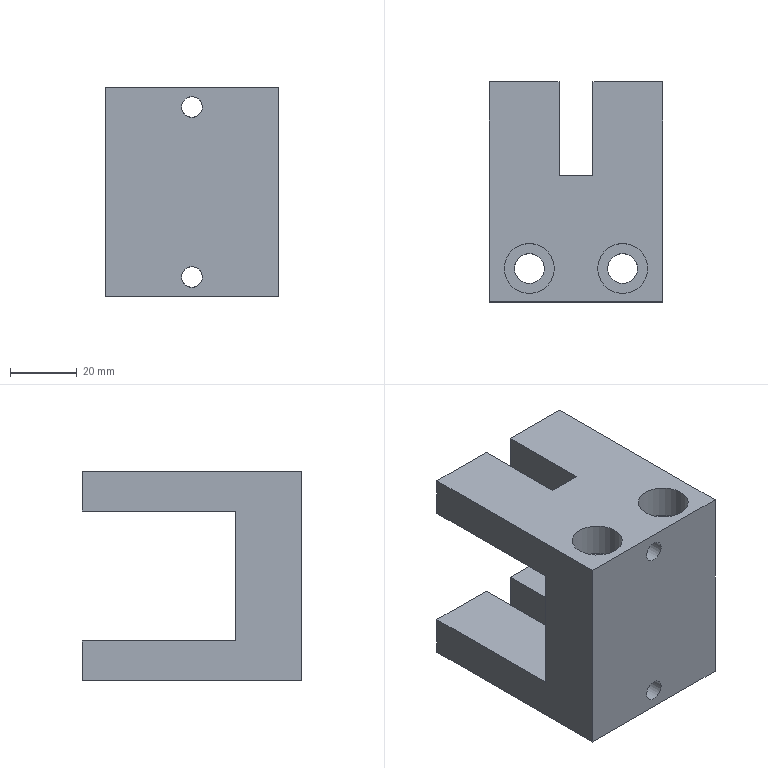Part | NX | 1 solid | 26 faces | box 52 x 66 x 63 mm | volume 103483 mm3 | plane 20 | cylinder 6 | commonest cylinder face diameters 6.2 x2 9 x2 15 x2
STEP:
#1=CARTESIAN_POINT('',(427.314,-68.057,-211.3));
#2=VERTEX_POINT('',#1);
#3=CARTESIAN_POINT('',(419.814,-68.057,-211.3));
#4=DIRECTION('',(0.,0.,1.));
#5=DIRECTION('',(1.,0.,0.));
#6=AXIS2_PLACEMENT_3D('',#3,#4,#5);
#7=CIRCLE('',#6,7.5);
#8=EDGE_CURVE('',#2,#2,#7,.T.);
#9=ORIENTED_EDGE('',*,*,#8,.T.);
#10=EDGE_LOOP('',(#9));
#11=FACE_BOUND('',#10,.T.);
#12=CARTESIAN_POINT('',(412.314,-68.057,-221.3));
#13=VERTEX_POINT('',#12);
#14=CARTESIAN_POINT('',(419.814,-68.057,-221.3));
#15=DIRECTION('',(0.,0.,1.));
#16=DIRECTION('',(-1.,0.,0.));
#17=AXIS2_PLACEMENT_3D('',#14,#15,#16);
#18=CIRCLE('',#17,7.5);
#19=EDGE_CURVE('',#13,#13,#18,.T.);
#20=ORIENTED_EDGE('',*,*,#19,.F.);
#21=EDGE_LOOP('',(#20));
#22=FACE_BOUND('',#21,.T.);
#23=CARTESIAN_POINT('',(419.814,-68.057,-211.3));
#24=DIRECTION('',(0.,0.,-1.));
#25=DIRECTION('',(1.,0.,0.));
#26=AXIS2_PLACEMENT_3D('',#23,#24,#25);
#27=CYLINDRICAL_SURFACE('',#26,7.5);
#28=ADVANCED_FACE('',(#11,#22),#27,.F.);
#29=ORIENTED_EDGE('',*,*,#19,.T.);
#30=EDGE_LOOP('',(#29));
#31=FACE_BOUND('',#30,.T.);
#32=CARTESIAN_POINT('',(415.314,-68.057,-221.3));
#33=VERTEX_POINT('',#32);
#34=CARTESIAN_POINT('',(419.814,-68.057,-221.3));
#35=DIRECTION('',(0.,0.,-1.));
#36=DIRECTION('',(-1.,0.,0.));
#37=AXIS2_PLACEMENT_3D('',#34,#35,#36);
#38=CIRCLE('',#37,4.5);
#39=EDGE_CURVE('',#33,#33,#38,.T.);
#40=ORIENTED_EDGE('',*,*,#39,.T.);
#41=EDGE_LOOP('',(#40));
#42=FACE_BOUND('',#41,.T.);
#43=CARTESIAN_POINT('',(391.814,-68.057,-221.3));
#44=DIRECTION('',(0.,0.,-1.));
#45=DIRECTION('',(1.,0.,0.));
#46=AXIS2_PLACEMENT_3D('',#43,#44,#45);
#47=PLANE('',#46);
#48=ADVANCED_FACE('',(#31,#42),#47,.F.);
#49=CARTESIAN_POINT('',(415.314,-68.057,-274.3));
#50=VERTEX_POINT('',#49);
#51=CARTESIAN_POINT('',(419.814,-68.057,-274.3));
#52=DIRECTION('',(0.,0.,1.));
#53=DIRECTION('',(-1.,0.,0.));
#54=AXIS2_PLACEMENT_3D('',#51,#52,#53);
#55=CIRCLE('',#54,4.5);
#56=EDGE_CURVE('',#50,#50,#55,.T.);
#57=ORIENTED_EDGE('',*,*,#56,.F.);
#58=EDGE_LOOP('',(#57));
#59=FACE_BOUND('',#58,.T.);
#60=ORIENTED_EDGE('',*,*,#39,.F.);
#61=EDGE_LOOP('',(#60));
#62=FACE_BOUND('',#61,.T.);
#63=CARTESIAN_POINT('',(419.814,-68.057,-211.3));
#64=DIRECTION('',(0.,0.,-1.));
#65=DIRECTION('',(1.,0.,0.));
#66=AXIS2_PLACEMENT_3D('',#63,#64,#65);
#67=CYLINDRICAL_SURFACE('',#66,4.5);
#68=ADVANCED_FACE('',(#59,#62),#67,.F.);
#69=CARTESIAN_POINT('',(384.314,-68.057,-211.3));
#70=VERTEX_POINT('',#69);
#71=CARTESIAN_POINT('',(391.814,-68.057,-211.3));
#72=DIRECTION('',(0.,0.,-1.));
#73=DIRECTION('',(-1.,0.,0.));
#74=AXIS2_PLACEMENT_3D('',#71,#72,#73);
#75=CIRCLE('',#74,7.5);
#76=EDGE_CURVE('',#70,#70,#75,.T.);
#77=ORIENTED_EDGE('',*,*,#76,.F.);
#78=EDGE_LOOP('',(#77));
#79=FACE_BOUND('',#78,.T.);
#80=CARTESIAN_POINT('',(384.314,-68.057,-221.3));
#81=VERTEX_POINT('',#80);
#82=CARTESIAN_POINT('',(391.814,-68.057,-221.3));
#83=DIRECTION('',(0.,0.,-1.));
#84=DIRECTION('',(-1.,0.,0.));
#85=AXIS2_PLACEMENT_3D('',#82,#83,#84);
#86=CIRCLE('',#85,7.5);
#87=EDGE_CURVE('',#81,#81,#86,.T.);
#88=ORIENTED_EDGE('',*,*,#87,.T.);
#89=EDGE_LOOP('',(#88));
#90=FACE_BOUND('',#89,.T.);
#91=CARTESIAN_POINT('',(391.814,-68.057,-211.3));
#92=DIRECTION('',(0.,0.,-1.));
#93=DIRECTION('',(-1.,0.,0.));
#94=AXIS2_PLACEMENT_3D('',#91,#92,#93);
#95=CYLINDRICAL_SURFACE('',#94,7.5);
#96=ADVANCED_FACE('',(#79,#90),#95,.F.);
#97=ORIENTED_EDGE('',*,*,#87,.F.);
#98=EDGE_LOOP('',(#97));
#99=FACE_BOUND('',#98,.T.);
#100=CARTESIAN_POINT('',(396.314,-68.057,-221.3));
#101=VERTEX_POINT('',#100);
#102=CARTESIAN_POINT('',(391.814,-68.057,-221.3));
#103=DIRECTION('',(0.,0.,1.));
#104=DIRECTION('',(1.,0.,0.));
#105=AXIS2_PLACEMENT_3D('',#102,#103,#104);
#106=CIRCLE('',#105,4.5);
#107=EDGE_CURVE('',#101,#101,#106,.T.);
#108=ORIENTED_EDGE('',*,*,#107,.F.);
#109=EDGE_LOOP('',(#108));
#110=FACE_BOUND('',#109,.T.);
#111=CARTESIAN_POINT('',(391.814,-68.057,-221.3));
#112=DIRECTION('',(0.,0.,-1.));
#113=DIRECTION('',(1.,0.,0.));
#114=AXIS2_PLACEMENT_3D('',#111,#112,#113);
#115=PLANE('',#114);
#116=ADVANCED_FACE('',(#99,#110),#115,.F.);
#117=CARTESIAN_POINT('',(387.314,-68.057,-274.3));
#118=VERTEX_POINT('',#117);
#119=CARTESIAN_POINT('',(391.814,-68.057,-274.3));
#120=DIRECTION('',(0.,0.,1.));
#121=DIRECTION('',(-1.,0.,0.));
#122=AXIS2_PLACEMENT_3D('',#119,#120,#121);
#123=CIRCLE('',#122,4.5);
#124=EDGE_CURVE('',#118,#118,#123,.T.);
#125=ORIENTED_EDGE('',*,*,#124,.F.);
#126=EDGE_LOOP('',(#125));
#127=FACE_BOUND('',#126,.T.);
#128=ORIENTED_EDGE('',*,*,#107,.T.);
#129=EDGE_LOOP('',(#128));
#130=FACE_BOUND('',#129,.T.);
#131=CARTESIAN_POINT('',(391.814,-68.057,-211.3));
#132=DIRECTION('',(0.,0.,-1.));
#133=DIRECTION('',(-1.,0.,0.));
#134=AXIS2_PLACEMENT_3D('',#131,#132,#133);
#135=CYLINDRICAL_SURFACE('',#134,4.5);
#136=ADVANCED_FACE('',(#127,#130),#135,.F.);
#137=CARTESIAN_POINT('',(431.814,-78.057,-274.3));
#138=VERTEX_POINT('',#137);
#139=CARTESIAN_POINT('',(431.814,-78.057,-211.3));
#140=VERTEX_POINT('',#139);
#141=CARTESIAN_POINT('',(431.814,-78.057,-217.3));
#142=DIRECTION('',(0.,0.,1.));
#143=VECTOR('',#142,1000.);
#144=LINE('',#141,#143);
#145=EDGE_CURVE('',#138,#140,#144,.T.);
#146=ORIENTED_EDGE('',*,*,#145,.F.);
#147=CARTESIAN_POINT('',(431.814,-12.057,-274.3));
#148=VERTEX_POINT('',#147);
#149=CARTESIAN_POINT('',(431.814,-34.899,-274.3));
#150=DIRECTION('',(0.,-1.,0.));
#151=VECTOR('',#150,1000.);
#152=LINE('',#149,#151);
#153=EDGE_CURVE('',#148,#138,#152,.T.);
#154=ORIENTED_EDGE('',*,*,#153,.F.);
#155=CARTESIAN_POINT('',(431.814,-12.057,-262.3));
#156=VERTEX_POINT('',#155);
#157=CARTESIAN_POINT('',(431.814,-12.057,-242.8));
#158=DIRECTION('',(0.,0.,1.));
#159=VECTOR('',#158,1000.);
#160=LINE('',#157,#159);
#161=EDGE_CURVE('',#148,#156,#160,.T.);
#162=ORIENTED_EDGE('',*,*,#161,.T.);
#163=CARTESIAN_POINT('',(431.814,-58.057,-262.3));
#164=VERTEX_POINT('',#163);
#165=CARTESIAN_POINT('',(431.814,-25.057,-262.3));
#166=DIRECTION('',(0.,1.,0.));
#167=VECTOR('',#166,1000.);
#168=LINE('',#165,#167);
#169=EDGE_CURVE('',#164,#156,#168,.T.);
#170=ORIENTED_EDGE('',*,*,#169,.F.);
#171=CARTESIAN_POINT('',(431.814,-58.057,-223.3));
#172=VERTEX_POINT('',#171);
#173=CARTESIAN_POINT('',(431.814,-58.057,-242.8));
#174=DIRECTION('',(0.,0.,-1.));
#175=VECTOR('',#174,1000.);
#176=LINE('',#173,#175);
#177=EDGE_CURVE('',#172,#164,#176,.T.);
#178=ORIENTED_EDGE('',*,*,#177,.F.);
#179=CARTESIAN_POINT('',(431.814,-12.057,-223.3));
#180=VERTEX_POINT('',#179);
#181=CARTESIAN_POINT('',(431.814,-26.107,-223.3));
#182=DIRECTION('',(0.,1.,0.));
#183=VECTOR('',#182,1000.);
#184=LINE('',#181,#183);
#185=EDGE_CURVE('',#172,#180,#184,.T.);
#186=ORIENTED_EDGE('',*,*,#185,.T.);
#187=CARTESIAN_POINT('',(431.814,-12.057,-211.3));
#188=VERTEX_POINT('',#187);
#189=CARTESIAN_POINT('',(431.814,-12.057,-242.8));
#190=DIRECTION('',(0.,0.,1.));
#191=VECTOR('',#190,1000.);
#192=LINE('',#189,#191);
#193=EDGE_CURVE('',#180,#188,#192,.T.);
#194=ORIENTED_EDGE('',*,*,#193,.T.);
#195=CARTESIAN_POINT('',(431.814,-34.899,-211.3));
#196=DIRECTION('',(0.,-1.,0.));
#197=VECTOR('',#196,1000.);
#198=LINE('',#195,#197);
#199=EDGE_CURVE('',#188,#140,#198,.T.);
#200=ORIENTED_EDGE('',*,*,#199,.T.);
#201=EDGE_LOOP('',(#146,#154,#162,#170,#178,#186,#194,#200));
#202=FACE_BOUND('',#201,.T.);
#203=CARTESIAN_POINT('',(431.814,-26.107,-217.3));
#204=DIRECTION('',(-1.,0.,0.));
#205=DIRECTION('',(0.,0.,-1.));
#206=AXIS2_PLACEMENT_3D('',#203,#204,#205);
#207=PLANE('',#206);
#208=ADVANCED_FACE('',(#202),#207,.F.);
#209=CARTESIAN_POINT('',(402.714,-40.157,-268.3));
#210=VERTEX_POINT('',#209);
#211=CARTESIAN_POINT('',(405.814,-40.157,-268.3));
#212=DIRECTION('',(0.,-1.,0.));
#213=DIRECTION('',(-1.,0.,0.));
#214=AXIS2_PLACEMENT_3D('',#211,#212,#213);
#215=CIRCLE('',#214,3.1);
#216=EDGE_CURVE('',#210,#210,#215,.T.);
#217=ORIENTED_EDGE('',*,*,#216,.F.);
#218=EDGE_LOOP('',(#217));
#219=FACE_BOUND('',#218,.T.);
#220=CARTESIAN_POINT('',(405.814,-78.057,-271.4));
#221=VERTEX_POINT('',#220);
#222=CARTESIAN_POINT('',(405.814,-78.057,-268.3));
#223=DIRECTION('',(0.,-1.,0.));
#224=DIRECTION('',(0.,0.,-1.));
#225=AXIS2_PLACEMENT_3D('',#222,#223,#224);
#226=CIRCLE('',#225,3.1);
#227=EDGE_CURVE('',#221,#221,#226,.T.);
#228=ORIENTED_EDGE('',*,*,#227,.T.);
#229=EDGE_LOOP('',(#228));
#230=FACE_BOUND('',#229,.T.);
#231=CARTESIAN_POINT('',(405.814,-30.057,-268.3));
#232=DIRECTION('',(0.,-1.,0.));
#233=DIRECTION('',(-1.,0.,0.));
#234=AXIS2_PLACEMENT_3D('',#231,#232,#233);
#235=CYLINDRICAL_SURFACE('',#234,3.1);
#236=ADVANCED_FACE('',(#219,#230),#235,.F.);
#237=CARTESIAN_POINT('',(402.714,-40.157,-217.3));
#238=VERTEX_POINT('',#237);
#239=CARTESIAN_POINT('',(405.814,-40.157,-217.3));
#240=DIRECTION('',(0.,-1.,0.));
#241=DIRECTION('',(-1.,0.,0.));
#242=AXIS2_PLACEMENT_3D('',#239,#240,#241);
#243=CIRCLE('',#242,3.1);
#244=EDGE_CURVE('',#238,#238,#243,.T.);
#245=ORIENTED_EDGE('',*,*,#244,.F.);
#246=EDGE_LOOP('',(#245));
#247=FACE_BOUND('',#246,.T.);
#248=CARTESIAN_POINT('',(405.814,-78.057,-220.4));
#249=VERTEX_POINT('',#248);
#250=CARTESIAN_POINT('',(405.814,-78.057,-217.3));
#251=DIRECTION('',(0.,-1.,0.));
#252=DIRECTION('',(0.,0.,-1.));
#253=AXIS2_PLACEMENT_3D('',#250,#251,#252);
#254=CIRCLE('',#253,3.1);
#255=EDGE_CURVE('',#249,#249,#254,.T.);
#256=ORIENTED_EDGE('',*,*,#255,.T.);
#257=EDGE_LOOP('',(#256));
#258=FACE_BOUND('',#257,.T.);
#259=CARTESIAN_POINT('',(405.814,-30.057,-217.3));
#260=DIRECTION('',(0.,-1.,0.));
#261=DIRECTION('',(-1.,0.,0.));
#262=AXIS2_PLACEMENT_3D('',#259,#260,#261);
#263=CYLINDRICAL_SURFACE('',#262,3.1);
#264=ADVANCED_FACE('',(#247,#258),#263,.F.);
#265=CARTESIAN_POINT('',(410.914,-40.157,-262.3));
#266=VERTEX_POINT('',#265);
#267=CARTESIAN_POINT('',(410.914,-40.157,-274.3));
#268=VERTEX_POINT('',#267);
#269=CARTESIAN_POINT('',(410.914,-40.157,-242.8));
#270=DIRECTION('',(0.,0.,-1.));
#271=VECTOR('',#270,1000.);
#272=LINE('',#269,#271);
#273=EDGE_CURVE('',#266,#268,#272,.T.);
#274=ORIENTED_EDGE('',*,*,#273,.T.);
#275=CARTESIAN_POINT('',(400.714,-40.157,-274.3));
#276=VERTEX_POINT('',#275);
#277=CARTESIAN_POINT('',(405.814,-40.157,-274.3));
#278=DIRECTION('',(1.,0.,0.));
#279=VECTOR('',#278,1000.);
#280=LINE('',#277,#279);
#281=EDGE_CURVE('',#276,#268,#280,.T.);
#282=ORIENTED_EDGE('',*,*,#281,.F.);
#283=CARTESIAN_POINT('',(400.714,-40.157,-262.3));
#284=VERTEX_POINT('',#283);
#285=CARTESIAN_POINT('',(400.714,-40.157,-242.8));
#286=DIRECTION('',(0.,0.,1.));
#287=VECTOR('',#286,1000.);
#288=LINE('',#285,#287);
#289=EDGE_CURVE('',#276,#284,#288,.T.);
#290=ORIENTED_EDGE('',*,*,#289,.T.);
#291=CARTESIAN_POINT('',(405.814,-40.157,-262.3));
#292=DIRECTION('',(-1.,0.,0.));
#293=VECTOR('',#292,1000.);
#294=LINE('',#291,#293);
#295=EDGE_CURVE('',#266,#284,#294,.T.);
#296=ORIENTED_EDGE('',*,*,#295,.F.);
#297=EDGE_LOOP('',(#274,#282,#290,#296));
#298=FACE_BOUND('',#297,.T.);
#299=ORIENTED_EDGE('',*,*,#216,.T.);
#300=EDGE_LOOP('',(#299));
#301=FACE_BOUND('',#300,.T.);
#302=CARTESIAN_POINT('',(400.714,-40.157,-242.8));
#303=DIRECTION('',(0.,-1.,0.));
#304=DIRECTION('',(-1.,0.,0.));
#305=AXIS2_PLACEMENT_3D('',#302,#303,#304);
#306=PLANE('',#305);
#307=ADVANCED_FACE('',(#298,#301),#306,.F.);
#308=ORIENTED_EDGE('',*,*,#289,.F.);
#309=CARTESIAN_POINT('',(400.714,-12.057,-274.3));
#310=VERTEX_POINT('',#309);
#311=CARTESIAN_POINT('',(400.714,-34.899,-274.3));
#312=DIRECTION('',(0.,-1.,0.));
#313=VECTOR('',#312,1000.);
#314=LINE('',#311,#313);
#315=EDGE_CURVE('',#310,#276,#314,.T.);
#316=ORIENTED_EDGE('',*,*,#315,.F.);
#317=CARTESIAN_POINT('',(400.714,-12.057,-262.3));
#318=VERTEX_POINT('',#317);
#319=CARTESIAN_POINT('',(400.714,-12.057,-242.8));
#320=DIRECTION('',(0.,0.,1.));
#321=VECTOR('',#320,1000.);
#322=LINE('',#319,#321);
#323=EDGE_CURVE('',#310,#318,#322,.T.);
#324=ORIENTED_EDGE('',*,*,#323,.T.);
#325=CARTESIAN_POINT('',(400.714,-25.057,-262.3));
#326=DIRECTION('',(0.,1.,0.));
#327=VECTOR('',#326,1000.);
#328=LINE('',#325,#327);
#329=EDGE_CURVE('',#284,#318,#328,.T.);
#330=ORIENTED_EDGE('',*,*,#329,.F.);
#331=EDGE_LOOP('',(#308,#316,#324,#330));
#332=FACE_BOUND('',#331,.T.);
#333=CARTESIAN_POINT('',(400.714,-25.057,-242.8));
#334=DIRECTION('',(-1.,0.,0.));
#335=DIRECTION('',(0.,1.,0.));
#336=AXIS2_PLACEMENT_3D('',#333,#334,#335);
#337=PLANE('',#336);
#338=ADVANCED_FACE('',(#332),#337,.F.);
#339=CARTESIAN_POINT('',(410.914,-12.057,-262.3));
#340=VERTEX_POINT('',#339);
#341=CARTESIAN_POINT('',(410.914,-12.057,-274.3));
#342=VERTEX_POINT('',#341);
#343=CARTESIAN_POINT('',(410.914,-12.057,-242.8));
#344=DIRECTION('',(0.,0.,-1.));
#345=VECTOR('',#344,1000.);
#346=LINE('',#343,#345);
#347=EDGE_CURVE('',#340,#342,#346,.T.);
#348=ORIENTED_EDGE('',*,*,#347,.T.);
#349=CARTESIAN_POINT('',(410.914,-34.899,-274.3));
#350=DIRECTION('',(0.,1.,0.));
#351=VECTOR('',#350,1000.);
#352=LINE('',#349,#351);
#353=EDGE_CURVE('',#268,#342,#352,.T.);
#354=ORIENTED_EDGE('',*,*,#353,.F.);
#355=ORIENTED_EDGE('',*,*,#273,.F.);
#356=CARTESIAN_POINT('',(410.914,-25.057,-262.3));
#357=DIRECTION('',(0.,-1.,0.));
#358=VECTOR('',#357,1000.);
#359=LINE('',#356,#358);
#360=EDGE_CURVE('',#340,#266,#359,.T.);
#361=ORIENTED_EDGE('',*,*,#360,.F.);
#362=EDGE_LOOP('',(#348,#354,#355,#361));
#363=FACE_BOUND('',#362,.T.);
#364=CARTESIAN_POINT('',(410.914,-25.057,-242.8));
#365=DIRECTION('',(1.,0.,0.));
#366=DIRECTION('',(0.,-1.,0.));
#367=AXIS2_PLACEMENT_3D('',#364,#365,#366);
#368=PLANE('',#367);
#369=ADVANCED_FACE('',(#363),#368,.F.);
#370=CARTESIAN_POINT('',(410.914,-40.157,-211.3));
#371=VERTEX_POINT('',#370);
#372=CARTESIAN_POINT('',(410.914,-12.057,-211.3));
#373=VERTEX_POINT('',#372);
#374=CARTESIAN_POINT('',(410.914,-34.899,-211.3));
#375=DIRECTION('',(0.,1.,0.));
#376=VECTOR('',#375,1000.);
#377=LINE('',#374,#376);
#378=EDGE_CURVE('',#371,#373,#377,.T.);
#379=ORIENTED_EDGE('',*,*,#378,.T.);
#380=CARTESIAN_POINT('',(410.914,-12.057,-223.3));
#381=VERTEX_POINT('',#380);
#382=CARTESIAN_POINT('',(410.914,-12.057,-242.8));
#383=DIRECTION('',(0.,0.,-1.));
#384=VECTOR('',#383,1000.);
#385=LINE('',#382,#384);
#386=EDGE_CURVE('',#373,#381,#385,.T.);
#387=ORIENTED_EDGE('',*,*,#386,.T.);
#388=CARTESIAN_POINT('',(410.914,-40.157,-223.3));
#389=VERTEX_POINT('',#388);
#390=CARTESIAN_POINT('',(410.914,-25.057,-223.3));
#391=DIRECTION('',(0.,1.,0.));
#392=VECTOR('',#391,1000.);
#393=LINE('',#390,#392);
#394=EDGE_CURVE('',#389,#381,#393,.T.);
#395=ORIENTED_EDGE('',*,*,#394,.F.);
#396=CARTESIAN_POINT('',(410.914,-40.157,-242.8));
#397=DIRECTION('',(0.,0.,-1.));
#398=VECTOR('',#397,1000.);
#399=LINE('',#396,#398);
#400=EDGE_CURVE('',#371,#389,#399,.T.);
#401=ORIENTED_EDGE('',*,*,#400,.F.);
#402=EDGE_LOOP('',(#379,#387,#395,#401));
#403=FACE_BOUND('',#402,.T.);
#404=CARTESIAN_POINT('',(410.914,-25.057,-242.8));
#405=DIRECTION('',(1.,0.,0.));
#406=DIRECTION('',(0.,-1.,0.));
#407=AXIS2_PLACEMENT_3D('',#404,#405,#406);
#408=PLANE('',#407);
#409=ADVANCED_FACE('',(#403),#408,.F.);
#410=CARTESIAN_POINT('',(400.714,-12.057,-211.3));
#411=VERTEX_POINT('',#410);
#412=CARTESIAN_POINT('',(400.714,-40.157,-211.3));
#413=VERTEX_POINT('',#412);
#414=CARTESIAN_POINT('',(400.714,-34.899,-211.3));
#415=DIRECTION('',(0.,-1.,0.));
#416=VECTOR('',#415,1000.);
#417=LINE('',#414,#416);
#418=EDGE_CURVE('',#411,#413,#417,.T.);
#419=ORIENTED_EDGE('',*,*,#418,.T.);
#420=CARTESIAN_POINT('',(400.714,-40.157,-223.3));
#421=VERTEX_POINT('',#420);
#422=CARTESIAN_POINT('',(400.714,-40.157,-242.8));
#423=DIRECTION('',(0.,0.,1.));
#424=VECTOR('',#423,1000.);
#425=LINE('',#422,#424);
#426=EDGE_CURVE('',#421,#413,#425,.T.);
#427=ORIENTED_EDGE('',*,*,#426,.F.);
#428=CARTESIAN_POINT('',(400.714,-12.057,-223.3));
#429=VERTEX_POINT('',#428);
#430=CARTESIAN_POINT('',(400.714,-25.057,-223.3));
#431=DIRECTION('',(0.,-1.,0.));
#432=VECTOR('',#431,1000.);
#433=LINE('',#430,#432);
#434=EDGE_CURVE('',#429,#421,#433,.T.);
#435=ORIENTED_EDGE('',*,*,#434,.F.);
#436=CARTESIAN_POINT('',(400.714,-12.057,-242.8));
#437=DIRECTION('',(0.,0.,1.));
#438=VECTOR('',#437,1000.);
#439=LINE('',#436,#438);
#440=EDGE_CURVE('',#429,#411,#439,.T.);
#441=ORIENTED_EDGE('',*,*,#440,.T.);
#442=EDGE_LOOP('',(#419,#427,#435,#441));
#443=FACE_BOUND('',#442,.T.);
#444=CARTESIAN_POINT('',(400.714,-25.057,-242.8));
#445=DIRECTION('',(-1.,0.,0.));
#446=DIRECTION('',(0.,1.,0.));
#447=AXIS2_PLACEMENT_3D('',#444,#445,#446);
#448=PLANE('',#447);
#449=ADVANCED_FACE('',(#443),#448,.F.);
#450=CARTESIAN_POINT('',(405.814,-40.157,-211.3));
#451=DIRECTION('',(1.,0.,0.));
#452=VECTOR('',#451,1000.);
#453=LINE('',#450,#452);
#454=EDGE_CURVE('',#413,#371,#453,.T.);
#455=ORIENTED_EDGE('',*,*,#454,.T.);
#456=ORIENTED_EDGE('',*,*,#400,.T.);
#457=CARTESIAN_POINT('',(405.814,-40.157,-223.3));
#458=DIRECTION('',(1.,0.,0.));
#459=VECTOR('',#458,1000.);
#460=LINE('',#457,#459);
#461=EDGE_CURVE('',#421,#389,#460,.T.);
#462=ORIENTED_EDGE('',*,*,#461,.F.);
#463=ORIENTED_EDGE('',*,*,#426,.T.);
#464=EDGE_LOOP('',(#455,#456,#462,#463));
#465=FACE_BOUND('',#464,.T.);
#466=ORIENTED_EDGE('',*,*,#244,.T.);
#467=EDGE_LOOP('',(#466));
#468=FACE_BOUND('',#467,.T.);
#469=CARTESIAN_POINT('',(400.714,-40.157,-242.8));
#470=DIRECTION('',(0.,-1.,0.));
#471=DIRECTION('',(-1.,0.,0.));
#472=AXIS2_PLACEMENT_3D('',#469,#470,#471);
#473=PLANE('',#472);
#474=ADVANCED_FACE('',(#465,#468),#473,.F.);
#475=CARTESIAN_POINT('',(379.814,-58.057,-223.3));
#476=VERTEX_POINT('',#475);
#477=CARTESIAN_POINT('',(405.814,-58.057,-223.3));
#478=DIRECTION('',(-1.,0.,0.));
#479=VECTOR('',#478,1000.);
#480=LINE('',#477,#479);
#481=EDGE_CURVE('',#172,#476,#480,.T.);
#482=ORIENTED_EDGE('',*,*,#481,.T.);
#483=CARTESIAN_POINT('',(379.814,-12.057,-223.3));
#484=VERTEX_POINT('',#483);
#485=CARTESIAN_POINT('',(379.814,-25.057,-223.3));
#486=DIRECTION('',(0.,-1.,0.));
#487=VECTOR('',#486,1000.);
#488=LINE('',#485,#487);
#489=EDGE_CURVE('',#484,#476,#488,.T.);
#490=ORIENTED_EDGE('',*,*,#489,.F.);
#491=CARTESIAN_POINT('',(405.814,-12.057,-223.3));
#492=DIRECTION('',(-1.,0.,0.));
#493=VECTOR('',#492,1000.);
#494=LINE('',#491,#493);
#495=EDGE_CURVE('',#429,#484,#494,.T.);
#496=ORIENTED_EDGE('',*,*,#495,.F.);
#497=ORIENTED_EDGE('',*,*,#434,.T.);
#498=ORIENTED_EDGE('',*,*,#461,.T.);
#499=ORIENTED_EDGE('',*,*,#394,.T.);
#500=CARTESIAN_POINT('',(405.814,-12.057,-223.3));
#501=DIRECTION('',(-1.,0.,0.));
#502=VECTOR('',#501,1000.);
#503=LINE('',#500,#502);
#504=EDGE_CURVE('',#180,#381,#503,.T.);
#505=ORIENTED_EDGE('',*,*,#504,.F.);
#506=ORIENTED_EDGE('',*,*,#185,.F.);
#507=EDGE_LOOP('',(#482,#490,#496,#497,#498,#499,#505,#506));
#508=FACE_BOUND('',#507,.T.);
#509=CARTESIAN_POINT('',(405.814,-25.057,-223.3));
#510=DIRECTION('',(0.,0.,1.));
#511=DIRECTION('',(1.,0.,0.));
#512=AXIS2_PLACEMENT_3D('',#509,#510,#511);
#513=PLANE('',#512);
#514=ADVANCED_FACE('',(#508),#513,.F.);
#515=ORIENTED_EDGE('',*,*,#440,.F.);
#516=ORIENTED_EDGE('',*,*,#495,.T.);
#517=CARTESIAN_POINT('',(379.814,-12.057,-211.3));
#518=VERTEX_POINT('',#517);
#519=CARTESIAN_POINT('',(379.814,-12.057,-242.8));
#520=DIRECTION('',(0.,0.,-1.));
#521=VECTOR('',#520,1000.);
#522=LINE('',#519,#521);
#523=EDGE_CURVE('',#518,#484,#522,.T.);
#524=ORIENTED_EDGE('',*,*,#523,.F.);
#525=CARTESIAN_POINT('',(405.814,-12.057,-211.3));
#526=DIRECTION('',(-1.,0.,0.));
#527=VECTOR('',#526,1000.);
#528=LINE('',#525,#527);
#529=EDGE_CURVE('',#411,#518,#528,.T.);
#530=ORIENTED_EDGE('',*,*,#529,.F.);
#531=EDGE_LOOP('',(#515,#516,#524,#530));
#532=FACE_BOUND('',#531,.T.);
#533=CARTESIAN_POINT('',(405.814,-12.057,-242.8));
#534=DIRECTION('',(0.,1.,0.));
#535=DIRECTION('',(1.,0.,0.));
#536=AXIS2_PLACEMENT_3D('',#533,#534,#535);
#537=PLANE('',#536);
#538=ADVANCED_FACE('',(#532),#537,.T.);
#539=ORIENTED_EDGE('',*,*,#323,.F.);
#540=CARTESIAN_POINT('',(379.814,-12.057,-274.3));
#541=VERTEX_POINT('',#540);
#542=CARTESIAN_POINT('',(405.814,-12.057,-274.3));
#543=DIRECTION('',(1.,0.,0.));
#544=VECTOR('',#543,1000.);
#545=LINE('',#542,#544);
#546=EDGE_CURVE('',#541,#310,#545,.T.);
#547=ORIENTED_EDGE('',*,*,#546,.F.);
#548=CARTESIAN_POINT('',(379.814,-12.057,-262.3));
#549=VERTEX_POINT('',#548);
#550=CARTESIAN_POINT('',(379.814,-12.057,-242.8));
#551=DIRECTION('',(0.,0.,-1.));
#552=VECTOR('',#551,1000.);
#553=LINE('',#550,#552);
#554=EDGE_CURVE('',#549,#541,#553,.T.);
#555=ORIENTED_EDGE('',*,*,#554,.F.);
#556=CARTESIAN_POINT('',(405.814,-12.057,-262.3));
#557=DIRECTION('',(1.,0.,0.));
#558=VECTOR('',#557,1000.);
#559=LINE('',#556,#558);
#560=EDGE_CURVE('',#549,#318,#559,.T.);
#561=ORIENTED_EDGE('',*,*,#560,.T.);
#562=EDGE_LOOP('',(#539,#547,#555,#561));
#563=FACE_BOUND('',#562,.T.);
#564=CARTESIAN_POINT('',(405.814,-12.057,-242.8));
#565=DIRECTION('',(0.,1.,0.));
#566=DIRECTION('',(1.,0.,0.));
#567=AXIS2_PLACEMENT_3D('',#564,#565,#566);
#568=PLANE('',#567);
#569=ADVANCED_FACE('',(#563),#568,.T.);
#570=CARTESIAN_POINT('',(405.814,-12.057,-262.3));
#571=DIRECTION('',(1.,0.,0.));
#572=VECTOR('',#571,1000.);
#573=LINE('',#570,#572);
#574=EDGE_CURVE('',#340,#156,#573,.T.);
#575=ORIENTED_EDGE('',*,*,#574,.F.);
#576=ORIENTED_EDGE('',*,*,#360,.T.);
#577=ORIENTED_EDGE('',*,*,#295,.T.);
#578=ORIENTED_EDGE('',*,*,#329,.T.);
#579=ORIENTED_EDGE('',*,*,#560,.F.);
#580=CARTESIAN_POINT('',(379.814,-58.057,-262.3));
#581=VERTEX_POINT('',#580);
#582=CARTESIAN_POINT('',(379.814,-25.057,-262.3));
#583=DIRECTION('',(0.,1.,0.));
#584=VECTOR('',#583,1000.);
#585=LINE('',#582,#584);
#586=EDGE_CURVE('',#581,#549,#585,.T.);
#587=ORIENTED_EDGE('',*,*,#586,.F.);
#588=CARTESIAN_POINT('',(405.814,-58.057,-262.3));
#589=DIRECTION('',(1.,0.,0.));
#590=VECTOR('',#589,1000.);
#591=LINE('',#588,#590);
#592=EDGE_CURVE('',#581,#164,#591,.T.);
#593=ORIENTED_EDGE('',*,*,#592,.T.);
#594=ORIENTED_EDGE('',*,*,#169,.T.);
#595=EDGE_LOOP('',(#575,#576,#577,#578,#579,#587,#593,#594));
#596=FACE_BOUND('',#595,.T.);
#597=CARTESIAN_POINT('',(405.814,-25.057,-262.3));
#598=DIRECTION('',(0.,0.,-1.));
#599=DIRECTION('',(1.,0.,0.));
#600=AXIS2_PLACEMENT_3D('',#597,#598,#599);
#601=PLANE('',#600);
#602=ADVANCED_FACE('',(#596),#601,.F.);
#603=ORIENTED_EDGE('',*,*,#592,.F.);
#604=CARTESIAN_POINT('',(379.814,-58.057,-242.8));
#605=DIRECTION('',(0.,0.,-1.));
#606=VECTOR('',#605,1000.);
#607=LINE('',#604,#606);
#608=EDGE_CURVE('',#476,#581,#607,.T.);
#609=ORIENTED_EDGE('',*,*,#608,.F.);
#610=ORIENTED_EDGE('',*,*,#481,.F.);
#611=ORIENTED_EDGE('',*,*,#177,.T.);
#612=EDGE_LOOP('',(#603,#609,#610,#611));
#613=FACE_BOUND('',#612,.T.);
#614=CARTESIAN_POINT('',(405.814,-58.057,-242.8));
#615=DIRECTION('',(0.,-1.,0.));
#616=DIRECTION('',(-1.,0.,0.));
#617=AXIS2_PLACEMENT_3D('',#614,#615,#616);
#618=PLANE('',#617);
#619=ADVANCED_FACE('',(#613),#618,.F.);
#620=CARTESIAN_POINT('',(379.814,-78.057,-274.3));
#621=VERTEX_POINT('',#620);
#622=CARTESIAN_POINT('',(405.814,-78.057,-274.3));
#623=DIRECTION('',(1.,0.,0.));
#624=VECTOR('',#623,1000.);
#625=LINE('',#622,#624);
#626=EDGE_CURVE('',#621,#138,#625,.T.);
#627=ORIENTED_EDGE('',*,*,#626,.F.);
#628=CARTESIAN_POINT('',(379.814,-34.899,-274.3));
#629=DIRECTION('',(0.,-1.,0.));
#630=VECTOR('',#629,1000.);
#631=LINE('',#628,#630);
#632=EDGE_CURVE('',#541,#621,#631,.T.);
#633=ORIENTED_EDGE('',*,*,#632,.F.);
#634=ORIENTED_EDGE('',*,*,#546,.T.);
#635=ORIENTED_EDGE('',*,*,#315,.T.);
#636=ORIENTED_EDGE('',*,*,#281,.T.);
#637=ORIENTED_EDGE('',*,*,#353,.T.);
#638=CARTESIAN_POINT('',(405.814,-12.057,-274.3));
#639=DIRECTION('',(1.,0.,0.));
#640=VECTOR('',#639,1000.);
#641=LINE('',#638,#640);
#642=EDGE_CURVE('',#342,#148,#641,.T.);
#643=ORIENTED_EDGE('',*,*,#642,.T.);
#644=ORIENTED_EDGE('',*,*,#153,.T.);
#645=EDGE_LOOP('',(#627,#633,#634,#635,#636,#637,#643,#644));
#646=FACE_BOUND('',#645,.T.);
#647=ORIENTED_EDGE('',*,*,#124,.T.);
#648=EDGE_LOOP('',(#647));
#649=FACE_BOUND('',#648,.T.);
#650=ORIENTED_EDGE('',*,*,#56,.T.);
#651=EDGE_LOOP('',(#650));
#652=FACE_BOUND('',#651,.T.);
#653=CARTESIAN_POINT('',(405.814,-34.899,-274.3));
#654=DIRECTION('',(0.,0.,1.));
#655=DIRECTION('',(1.,0.,0.));
#656=AXIS2_PLACEMENT_3D('',#653,#654,#655);
#657=PLANE('',#656);
#658=ADVANCED_FACE('',(#646,#649,#652),#657,.F.);
#659=ORIENTED_EDGE('',*,*,#199,.F.);
#660=CARTESIAN_POINT('',(405.814,-12.057,-211.3));
#661=DIRECTION('',(-1.,0.,0.));
#662=VECTOR('',#661,1000.);
#663=LINE('',#660,#662);
#664=EDGE_CURVE('',#188,#373,#663,.T.);
#665=ORIENTED_EDGE('',*,*,#664,.T.);
#666=ORIENTED_EDGE('',*,*,#378,.F.);
#667=ORIENTED_EDGE('',*,*,#454,.F.);
#668=ORIENTED_EDGE('',*,*,#418,.F.);
#669=ORIENTED_EDGE('',*,*,#529,.T.);
#670=CARTESIAN_POINT('',(379.814,-78.057,-211.3));
#671=VERTEX_POINT('',#670);
#672=CARTESIAN_POINT('',(379.814,-34.899,-211.3));
#673=DIRECTION('',(0.,-1.,0.));
#674=VECTOR('',#673,1000.);
#675=LINE('',#672,#674);
#676=EDGE_CURVE('',#518,#671,#675,.T.);
#677=ORIENTED_EDGE('',*,*,#676,.T.);
#678=CARTESIAN_POINT('',(390.814,-78.057,-211.3));
#679=DIRECTION('',(-1.,0.,0.));
#680=VECTOR('',#679,1000.);
#681=LINE('',#678,#680);
#682=EDGE_CURVE('',#140,#671,#681,.T.);
#683=ORIENTED_EDGE('',*,*,#682,.F.);
#684=EDGE_LOOP('',(#659,#665,#666,#667,#668,#669,#677,#683));
#685=FACE_BOUND('',#684,.T.);
#686=ORIENTED_EDGE('',*,*,#76,.T.);
#687=EDGE_LOOP('',(#686));
#688=FACE_BOUND('',#687,.T.);
#689=ORIENTED_EDGE('',*,*,#8,.F.);
#690=EDGE_LOOP('',(#689));
#691=FACE_BOUND('',#690,.T.);
#692=CARTESIAN_POINT('',(405.814,-34.899,-211.3));
#693=DIRECTION('',(0.,0.,-1.));
#694=DIRECTION('',(-1.,0.,0.));
#695=AXIS2_PLACEMENT_3D('',#692,#693,#694);
#696=PLANE('',#695);
#697=ADVANCED_FACE('',(#685,#688,#691),#696,.F.);
#698=ORIENTED_EDGE('',*,*,#193,.F.);
#699=ORIENTED_EDGE('',*,*,#504,.T.);
#700=ORIENTED_EDGE('',*,*,#386,.F.);
#701=ORIENTED_EDGE('',*,*,#664,.F.);
#702=EDGE_LOOP('',(#698,#699,#700,#701));
#703=FACE_BOUND('',#702,.T.);
#704=CARTESIAN_POINT('',(405.814,-12.057,-242.8));
#705=DIRECTION('',(0.,1.,0.));
#706=DIRECTION('',(1.,0.,0.));
#707=AXIS2_PLACEMENT_3D('',#704,#705,#706);
#708=PLANE('',#707);
#709=ADVANCED_FACE('',(#703),#708,.T.);
#710=ORIENTED_EDGE('',*,*,#161,.F.);
#711=ORIENTED_EDGE('',*,*,#642,.F.);
#712=ORIENTED_EDGE('',*,*,#347,.F.);
#713=ORIENTED_EDGE('',*,*,#574,.T.);
#714=EDGE_LOOP('',(#710,#711,#712,#713));
#715=FACE_BOUND('',#714,.T.);
#716=CARTESIAN_POINT('',(405.814,-12.057,-242.8));
#717=DIRECTION('',(0.,1.,0.));
#718=DIRECTION('',(1.,0.,0.));
#719=AXIS2_PLACEMENT_3D('',#716,#717,#718);
#720=PLANE('',#719);
#721=ADVANCED_FACE('',(#715),#720,.T.);
#722=CARTESIAN_POINT('',(379.814,-78.057,-242.8));
#723=DIRECTION('',(0.,0.,-1.));
#724=VECTOR('',#723,1000.);
#725=LINE('',#722,#724);
#726=EDGE_CURVE('',#671,#621,#725,.T.);
#727=ORIENTED_EDGE('',*,*,#726,.F.);
#728=ORIENTED_EDGE('',*,*,#676,.F.);
#729=ORIENTED_EDGE('',*,*,#523,.T.);
#730=ORIENTED_EDGE('',*,*,#489,.T.);
#731=ORIENTED_EDGE('',*,*,#608,.T.);
#732=ORIENTED_EDGE('',*,*,#586,.T.);
#733=ORIENTED_EDGE('',*,*,#554,.T.);
#734=ORIENTED_EDGE('',*,*,#632,.T.);
#735=EDGE_LOOP('',(#727,#728,#729,#730,#731,#732,#733,#734));
#736=FACE_BOUND('',#735,.T.);
#737=CARTESIAN_POINT('',(379.814,-25.057,-242.8));
#738=DIRECTION('',(-1.,0.,0.));
#739=DIRECTION('',(0.,1.,0.));
#740=AXIS2_PLACEMENT_3D('',#737,#738,#739);
#741=PLANE('',#740);
#742=ADVANCED_FACE('',(#736),#741,.T.);
#743=ORIENTED_EDGE('',*,*,#227,.F.);
#744=EDGE_LOOP('',(#743));
#745=FACE_BOUND('',#744,.T.);
#746=ORIENTED_EDGE('',*,*,#255,.F.);
#747=EDGE_LOOP('',(#746));
#748=FACE_BOUND('',#747,.T.);
#749=ORIENTED_EDGE('',*,*,#145,.T.);
#750=ORIENTED_EDGE('',*,*,#682,.T.);
#751=ORIENTED_EDGE('',*,*,#726,.T.);
#752=ORIENTED_EDGE('',*,*,#626,.T.);
#753=EDGE_LOOP('',(#749,#750,#751,#752));
#754=FACE_BOUND('',#753,.T.);
#755=CARTESIAN_POINT('',(390.814,-78.057,-242.8));
#756=DIRECTION('',(0.,-1.,0.));
#757=DIRECTION('',(-1.,0.,0.));
#758=AXIS2_PLACEMENT_3D('',#755,#756,#757);
#759=PLANE('',#758);
#760=ADVANCED_FACE('',(#745,#748,#754),#759,.T.);
#761=CLOSED_SHELL('',(#28,#48,#68,#96,#116,#136,#208,#236,#264,#307,#338,#369,#409,#449,#474,#514,#538,#569,#602,#619,#658,#697,#709,#721,#742,#760));
#762=MANIFOLD_SOLID_BREP('',#761);
#763=(LENGTH_UNIT()NAMED_UNIT(*)SI_UNIT(.MILLI.,.METRE.));
#764=UNCERTAINTY_MEASURE_WITH_UNIT(LENGTH_MEASURE(0.00001),#763,'','');
#765=(NAMED_UNIT(*)PLANE_ANGLE_UNIT()SI_UNIT($,.RADIAN.));
#766=(NAMED_UNIT(*)SI_UNIT($,.STERADIAN.)SOLID_ANGLE_UNIT());
#767=(GEOMETRIC_REPRESENTATION_CONTEXT(3)GLOBAL_UNCERTAINTY_ASSIGNED_CONTEXT((#764))GLOBAL_UNIT_ASSIGNED_CONTEXT((#763,#765,#766))REPRESENTATION_CONTEXT('',''));
#768=ADVANCED_BREP_SHAPE_REPRESENTATION('',(#762),#767);